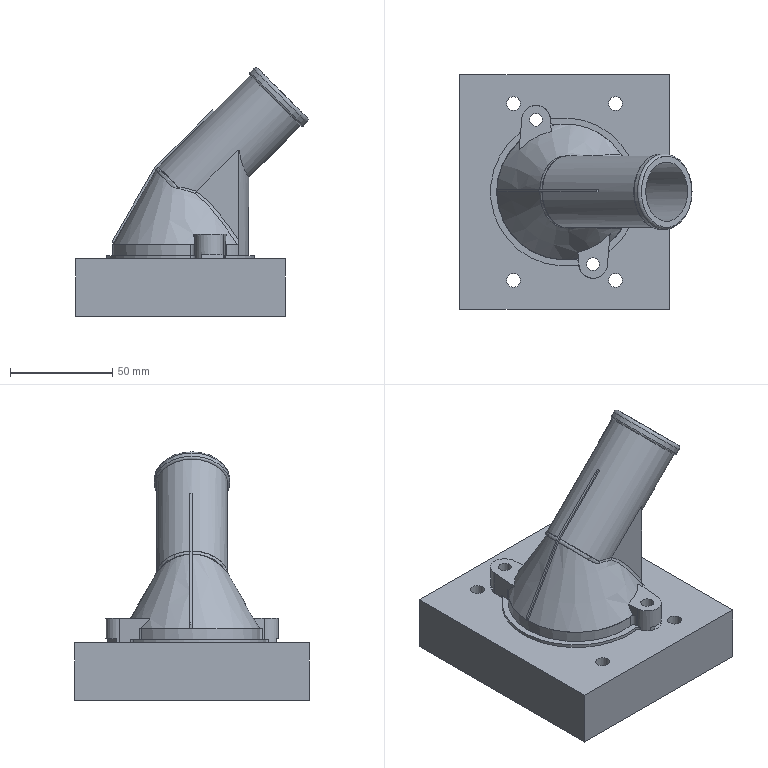NC program | NX | posted by the shop | part box 113.679 x 114.654 x 121.568 mm
Lines 24174 to 24444 of 160120:
24173 TOOL CALL Z S8000
24174 M3
24175 CYCL DEF 32.0 TOLERANCE
24176 CYCL DEF 32.1 T0.012
24177 CYCL DEF 32.2 HSC-MODE:0
24178 PLANE SPATIAL SPA-90. SPB+0.0 SPC+180. TURN FMAX SEQ-
24179 L X36.1116 Y-19.3551 FMAX
24180 L Z97.627 FMAX
24181 L Z.1 FMAX
24182 L X33.7116 F250.
24183 L X32.8138 F700.
24184 L X14.3856 Y-51.2733
24185 L X14.3016 Y-51.6013
24186 CC X10.4281 Y-50.2478
24187 C X12.1842 Y-53.9561 DR-
24188 L X-16.2168 Y-82.3572
24189 L X-17.9139 Y-84.0542
24190 L Z97.627 FMAX
24191 PLANE RESET STAY
24192 * - OPERATION: 新底壁铣_1_COPY - TOOL: T12 C-D4
24193 CALL LBL101
24194 CYCL DEF 32.0 TOLERANCE
24195 CYCL DEF 32.1 T0.012
24196 CYCL DEF 32.2 HSC-MODE:0
24197 PLANE SPATIAL SPA-90. SPB+0.0 SPC+0.0 TURN FMAX SEQ-
24198 L X17.9381 Y-84.0299 FMAX
24199 L Z97.627 FMAX
24200 L Z1.1 FMAX
24201 L X16.241 Y-82.3328 F250.
24202 L X-12.1582 Y-53.9335 F700.
24203 L X-12.6991 Y-53.6332
24204 CC X-10.3929 Y-50.2467
24205 C X-14.3764 Y-51.2053 DR-
24206 L X-25.957 Y-31.1877
24207 L X-28.7325 Y-26.3843
24208 L X-28.98 Y-26.126
24209 L X-29.4408 Y-25.5763
24210 CC X-20.4422 Y-18.7458
24211 C X-31.2553 Y-22.0181 DR-
24212 L X-32.8368 Y-19.2808
24213 L X-33.7545
24214 L X-36.1545
24215 L Z97.627 FMAX
24216 PLANE RESET STAY
24217 * - OPERATION: 新底壁铣_1_COPY_COPY - TOOL: T12 C-D4
24218 CALL LBL101
24219 CYCL DEF 32.0 TOLERANCE
24220 CYCL DEF 32.1 T0.012
24221 CYCL DEF 32.2 HSC-MODE:0
24222 PLANE SPATIAL SPA-59.979 SPB+0.0 SPC+90. TURN FMAX SEQ-
24223 L X5.4 Y-18.4254 FMAX
24224 L Z134.3072 FMAX
24225 L Y-18.4253 Z36.9726 FMAX
24226 L X3. F250.
24227 L Y-40.4123 F700.
24228 L X-2.
24229 L Y3.5617
24230 L X3.
24231 L Y-18.4253
24232 L X1.
24233 L Y-38.4123
24234 L X+0.0
24235 L Y1.5617
24236 L X1.
24237 L Y-18.4253
24238 L X3.4
24239 L Z134.3073 FMAX
24240 PLANE RESET STAY
24241 * - OPERATION: 新底壁铣_1_COPY_COPY_COPY - TOOL: T12 C-D4
24242 CALL LBL101
24243 CYCL DEF 32.0 TOLERANCE
24244 CYCL DEF 32.1 T0.012
24245 CYCL DEF 32.2 HSC-MODE:0
24246 PLANE SPATIAL SPA-44.957 SPB+0.0 SPC+90. TURN FMAX SEQ-
24247 L X5.4 Y-47.6035 FMAX
24248 L Z153.0518 FMAX
24249 L Y-47.6034 Z45.6685 FMAX
24250 L X3. F250.
24251 L Y-69.6641 F700.
24252 L X-2.
24253 L Y-25.5428
24254 L X3.
24255 L Y-47.6034
24256 L X1.
24257 L Y-67.6641
24258 L X+0.0
24259 L Y-27.5428
24260 L X1.
24261 L Y-47.6034
24262 L X3.4
24263 L Z153.0518 FMAX
24264 PLANE RESET STAY
24265 M50
24266 * - OPERATION: 2D光侧面 - TOOL: T15 J-D10
24267 M5
24268 M9
24269 PLANE RESET STAY
24270 CALL LBL100
24271 ;(J-D10 D=10. R=0.)
24272 M01
24273 TOOL CALL 15 Z S7000
24274 CALL LBL101
24275 M3 M8
24276 M51
24277 CYCL DEF 32.0 TOLERANCE
24278 CYCL DEF 32.1 T0.036
24279 CYCL DEF 32.2 HSC-MODE:0
24280 L M126
24281 PLANE SPATIAL SPA-90. SPB+0.0 SPC+180. TURN FMAX SEQ-
24282 L X39.2478 Y-15.013 FMAX
24283 L Z97.327 FMAX
24284 L Z.5 FMAX
24285 L Z+0.0 F250.
24286 CC X38.9214 Y-15.9583
24287 C X37.9762 Y-15.6319 DR+
24288 CC X33.25 Y-14.
24289 C X37.5801 Y-16.5 DR- F400.
24290 L X16.9014 Y-52.3167
24291 CC X10.3561 Y-50.2022
24292 C X13.8352 Y-56.1357 DR-
24293 L X-16.2207 Y-86.1836
24294 CC X-15.5136 Y-86.8908
24295 C X-16.2208 Y-87.5978 DR+
24296 L Z.5
24297 L Z97.327 FMAX
24298 PLANE RESET STAY
24299 * - OPERATION: 2D光侧面_COPY - TOOL: T15 J-D10
24300 CALL LBL101
24301 CYCL DEF 32.0 TOLERANCE
24302 CYCL DEF 32.1 T0.036
24303 CYCL DEF 32.2 HSC-MODE:0
24304 PLANE SPATIAL SPA-90. SPB+0.0 SPC+0.0 TURN FMAX SEQ-
24305 L X16.2427 Y-87.5756 FMAX
24306 L Z97.327 FMAX
24307 L Z1.5 FMAX
24308 L Z1. F250.
24309 CC X15.5356 Y-86.8685
24310 C X16.2427 Y-86.1614 DR+
24311 L X-13.8372 Y-56.0814 F400.
24312 L X-14.764 Y-55.4987
24313 L X-16.0288 Y-54.1236
24314 L X-16.7592 Y-52.7043
24315 L X-16.8735 Y-52.2951
24316 L X-37.5638 Y-16.5023
24317 CC X-33.2349 Y-14.
24318 C X-37.9753 Y-15.5903 DR-
24319 CC X-38.9234 Y-15.9083
24320 C X-39.2414 Y-14.9603 DR+
24321 L Z1.5
24322 L Z97.327 FMAX
24323 PLANE RESET STAY
24324 * - OPERATION: 新底壁铣_2 - TOOL: T15 J-D10
24325 CALL LBL101
24326 CYCL DEF 32.0 TOLERANCE
24327 CYCL DEF 32.1 T0.012
24328 CYCL DEF 32.2 HSC-MODE:0
24329 L A+0.0 C+0.0 FMAX
24330 L X8.8901 Y-47.7322 FMAX
24331 L Z160.5681 FMAX
24332 L Z8.5 FMAX
24333 L X4.95 Y-43.2072 F250.
24334 CC X14. Y-35.327
24335 C X2.3436 Y-38.1781 DR- F400.
24336 CC X+0.0 Y+0.0
24337 C X-37.8702 Y-5.3767 DR-
24338 CC X+0.0 Y+0.0
24339 C X-37.9218 Y-5. DR-
24340 L X-38.285
24341 L Y6.
24342 L X-37.7765
24343 CC X+0.0 Y+0.0
24344 C X-26.7148 Y27.3748 DR-
24345 L X-26.3319 Y31.7521
24346 L X-26.0704 Y34.7407
24347 L Z160.5681 FMAX
24348 PLANE RESET STAY
24349 * - OPERATION: 新底壁铣_2_COPY - TOOL: T15 J-D10
24350 CYCL DEF 32.0 TOLERANCE
24351 CYCL DEF 32.1 T0.012
24352 CYCL DEF 32.2 HSC-MODE:0
24353 L A+0.0 C+0.0 FMAX
24354 L X-31.9998 Y35.8099 FMAX
24355 L Z160.5681 FMAX
24356 L Z19. FMAX
24357 L X-26.0226 Y35.287 F250.
24358 L X-25.9974 Y35.5745 F400.
24359 CC X-14. Y35.327
24360 C X-2.0026 Y35.5745 DR-
24361 L X-1.9767 Y35.2791
24362 CC X-.0513 Y.0422
24363 C X-27.1147 Y22.6899 DR+
24364 L X-26.0226 Y35.287
24365 L X-21.0416 Y34.8512
24366 L X-21.0019 Y35.3048
24367 CC X-14.002 Y35.327
24368 C X-14. Y42.327 DR-
24369 CC X-14. Y35.327
24370 C X-8.3546 Y39.4658 DR-
24371 CC X-.1956 Y.4641
24372 C X-21.0813 Y34.3977 DR+
24373 L X-21.0416 Y34.8512
24374 L X-27.0188 Y35.3742
24375 L Z160.5681 FMAX
24376 L X31.9975 Y-35.8364 FMAX
24377 L Z19. FMAX
24378 L X26.0203 Y-35.3134 F250.
24379 L X25.9974 Y-35.5745 F400.
24380 CC X14. Y-35.327
24381 C X2.0026 Y-35.5745 DR-
24382 L X1.9836 Y-35.3581
24383 L X4.018 Y-35.1561
24384 L X4.8 Y-35.0686
24385 L X5.5857 Y-34.9422
24386 L X6.369 Y-34.8063
24387 L X7.4603 Y-34.5999
24388 L X7.551 Y-34.5827
24389 CC X-.3703 Y.8524
24390 C X18.121 Y-30.3961 DR+
24391 CC X-.5462 Y.6792
24392 C X22.8214 Y-27.0353 DR+
24393 L X23.457 Y-26.4948
24394 L X24.4913 Y-27.0294
24395 L X26.6559 Y-28.0481
24396 L X26.0203 Y-35.3134
24397 L X21.0393 Y-34.8777
24398 L X21.0019 Y-35.3048
24399 CC X14.002 Y-35.327
24400 C X14. Y-42.327 DR-
24401 CC X14. Y-35.327
24402 C X8.3894 Y-39.5129 DR-
24403 L X8.5596 Y-39.4807
24404 CC X-.3705 Y.8523
24405 C X20.6812 Y-34.691 DR+
24406 CC X-.5464 Y.6791
24407 C X21.0767 Y-34.4506 DR+
24408 L X21.0393 Y-34.8777
24409 L X27.0165 Y-35.4006
24410 L Z160.5681 FMAX
24411 PLANE RESET STAY
24412 M50
24413 * - OPERATION: 新底壁铣 - TOOL: T5 J-D10R0.5
24414 M5
24415 M9
24416 PLANE RESET STAY
24417 CALL LBL100
24418 ;(J-D10R0.5 D=10. R=0.5)
24419 M01
24420 TOOL CALL 5 Z S7000
24421 CALL LBL101
24422 M3 M8
24423 M51
24424 CYCL DEF 32.0 TOLERANCE
24425 CYCL DEF 32.1 T0.012
24426 CYCL DEF 32.2 HSC-MODE:0
24427 L M126
24428 PLANE SPATIAL SPA-45. SPB+0.0 SPC-90. TURN FMAX SEQ-
24429 L X-28.5 Y-26.9686 FMAX
24430 L Z171.5197 FMAX
24431 L Z97.6563 FMAX
24432 L X-22.5 F700.
24433 CC X+0.0 Y-26.9686
24434 C X-22.5 Y-26.9686 DR-
24435 L X-17.5
24436 CC X+0.0 Y-26.9686
24437 C X-17.5 Y-26.9686 DR-
24438 L X-12.5
24439 CC X+0.0 Y-26.9686
24440 C X-12.5 Y-26.9686 DR-
24441 L X-18.5
24442 L Z171.5197 FMAX
24443 PLANE RESET STAY